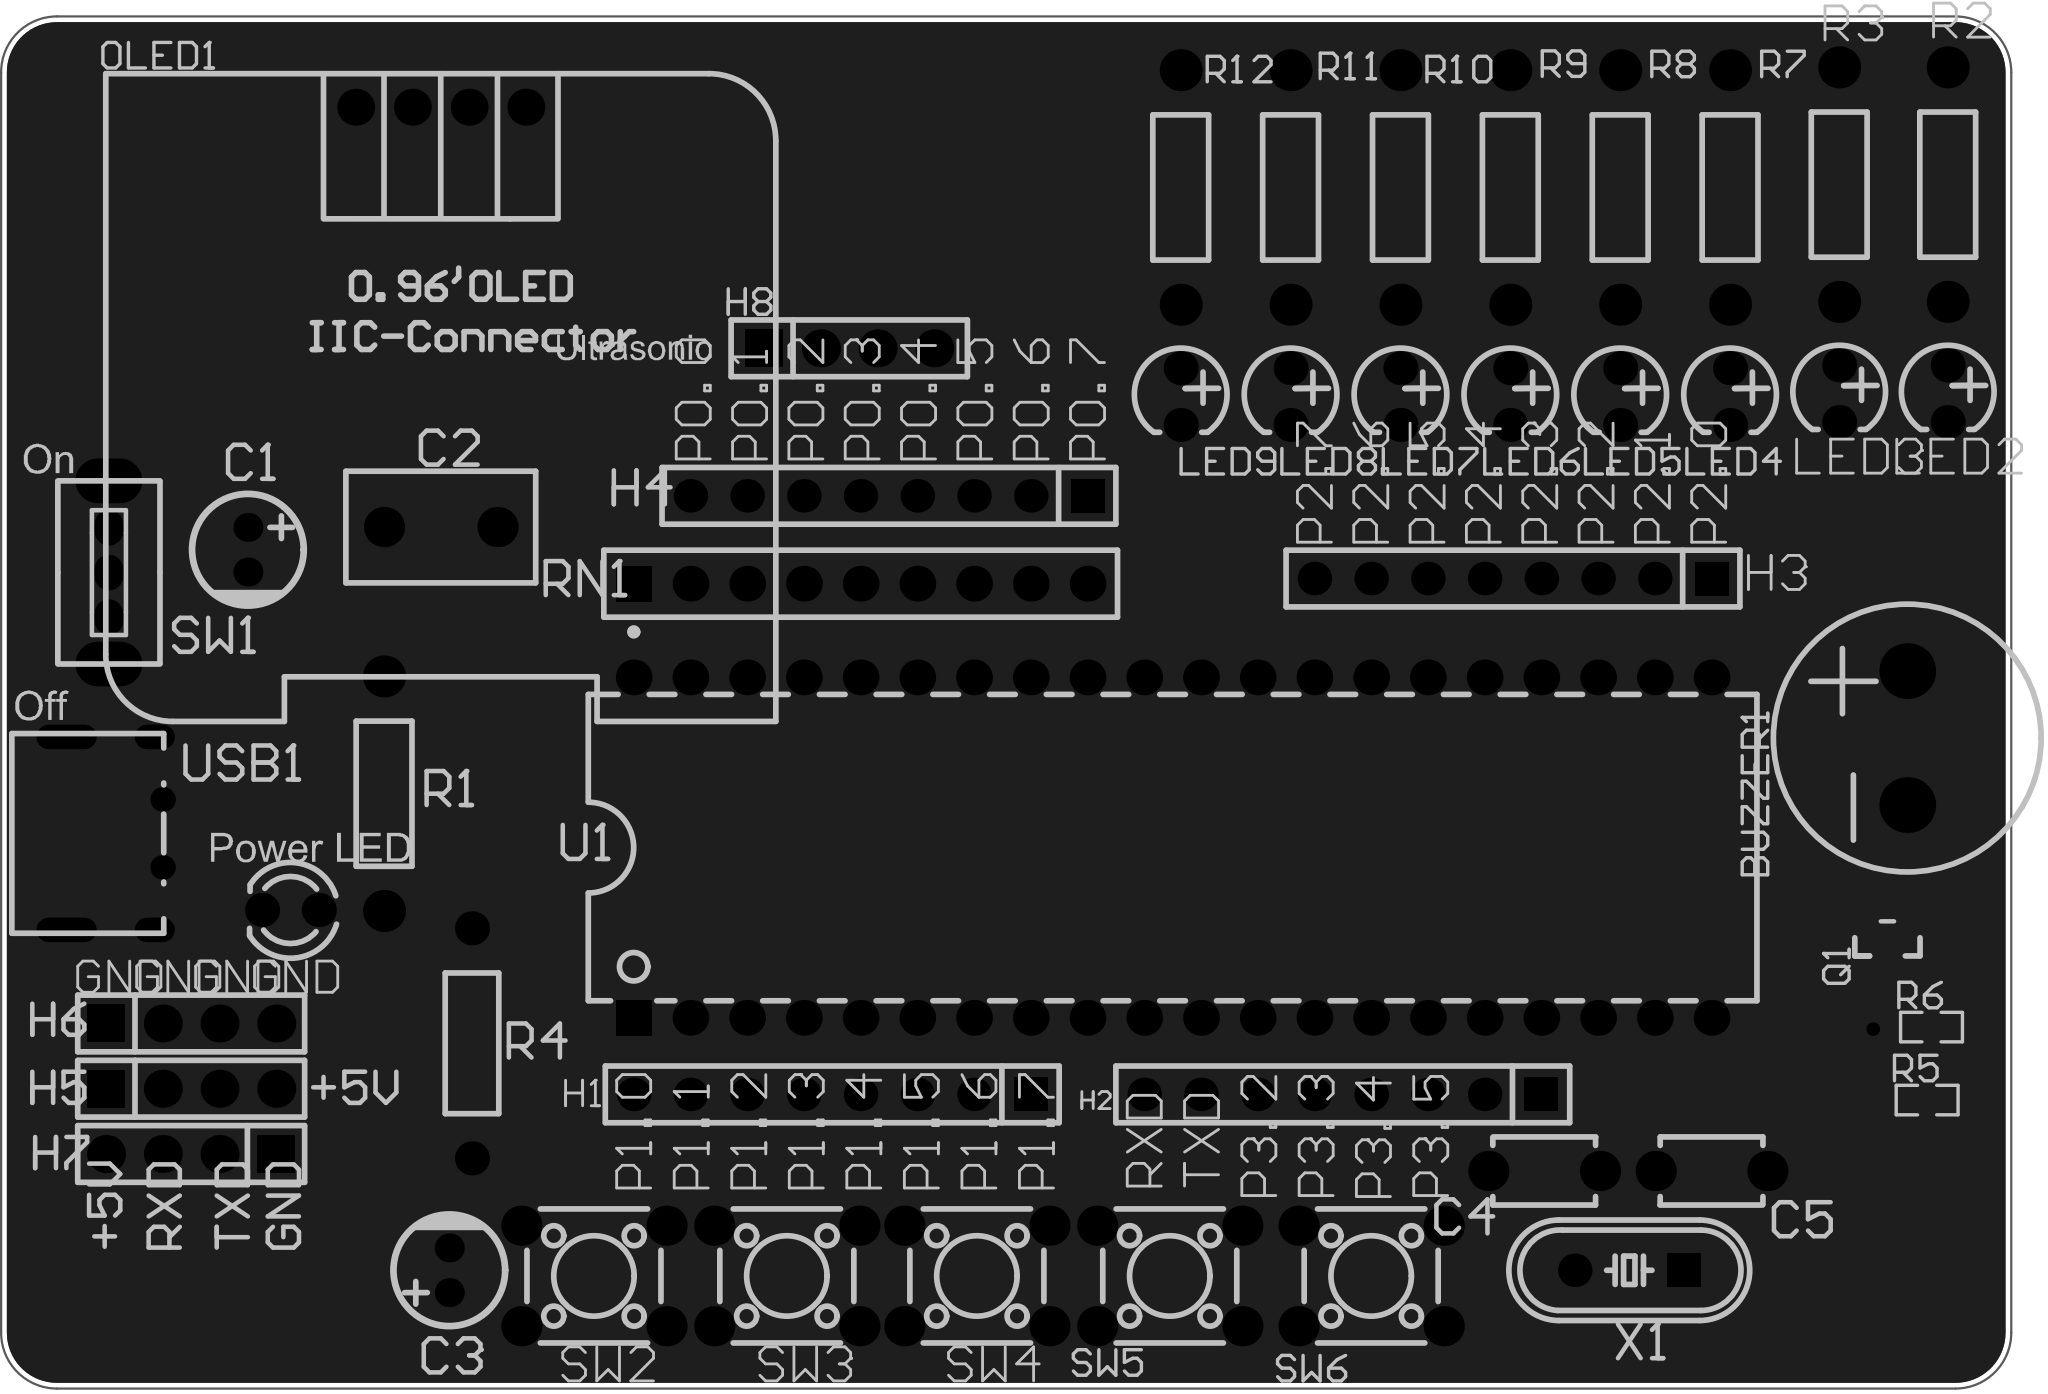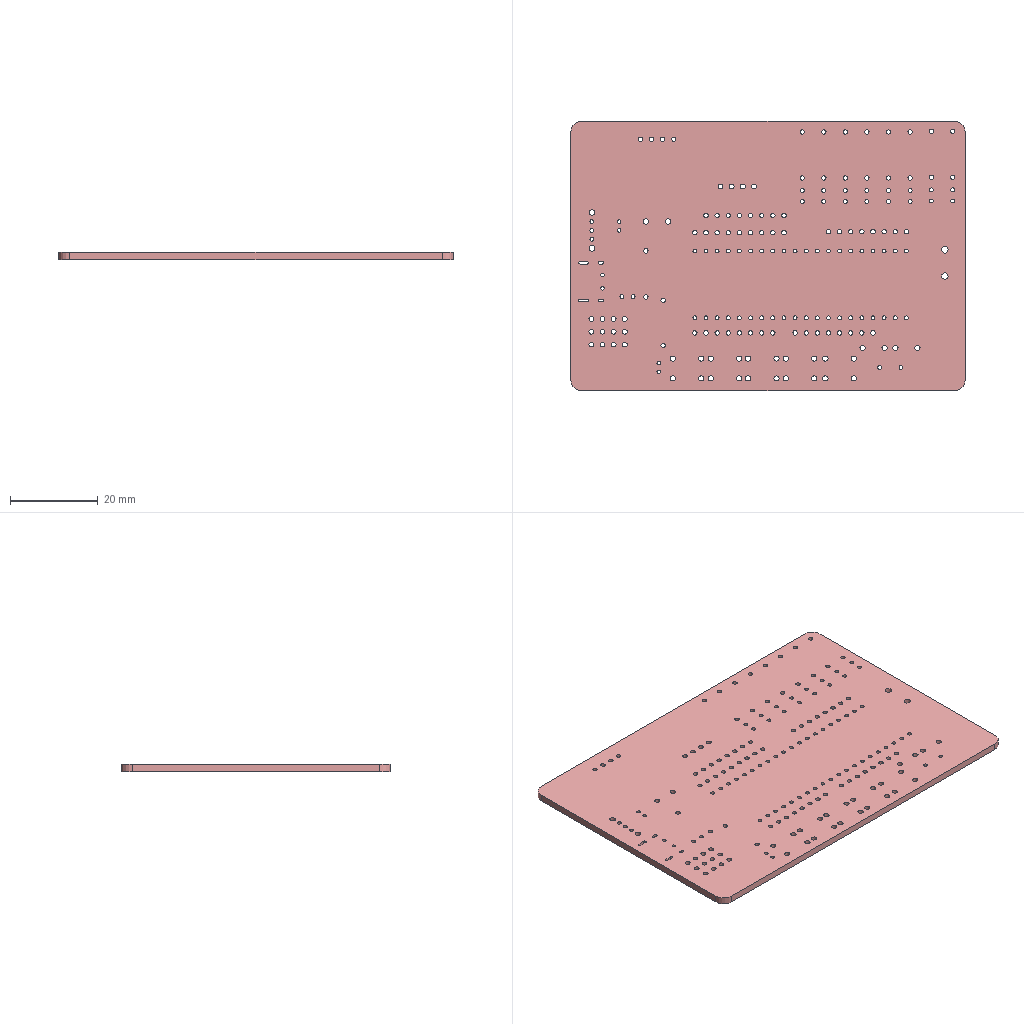Circuit board layout | Altium Designer | box 90 x 61.4 x 1.6 mm
Layer stack:
# Altium Designer layer stack of  (unit mm; dielectric type: 0 none, 1 core, 2 prepreg, 3 surface material)
index,name,kind,layer,copper_thickness_mm,dielectric_type,dielectric_thickness_mm,dielectric_material,dielectric_constant
0,Top Paste Mask Layer,other,,,,,,
1,Top Silkscreen Layer,other,,,,,,
2,Top Solder Mask Layer,dielectric,,,3,0.01,,3.3
3,Top Layer,copper,Top Layer,0.035,,,,
4,Dielectric1,dielectric,,,3,1.51,FR4,4.5
5,Bottom Layer,copper,Bottom Layer,0.035,,,,
6,Bottom Solder Mask Layer,dielectric,,,3,0.01,,3.3
7,Bottom Silkscreen Layer,other,,,,,,
8,Bottom Paste Mask Layer,other,,,,,,
# drill layer pairs: low layer,high layer
drill_pair,Top Layer,Bottom Layer
Part placement:
Designator,Comment,Layer,Footprint,Center-X(mm),Center-Y(mm),Rotation
U1,STC89C52RC-40I-PDIP40,TopLayer,DIP-40_L52.0-W13.7-P2.54-LS15.2-BL,128.651,100.457,0
SW3,,TopLayer,SW-TH_4P-L6.0-W6.0-P4.50-LS6.5,111.379,81.28,0
H8,,TopLayer,HDR-TH_4P-P2.54-V-F,114.173,122.809,0
SW4,,TopLayer,SW-TH_4P-L6.0-W6.0-P4.50-LS6.5,119.888,81.28,0
SW2,,TopLayer,SW-TH_4P-L6.0-W6.0-P4.50-LS6.5,102.743,81.28,180
RN1,10kΩ,TopLayer,RES-ARRAY-TH_9P-P2.54-D1.0,114.685,112.272,0
USB1,TYPE-C-31-M-33,TopLayer,USB-C-TH_TYPE-C-31-M-33,81.28,101.092,270
SW1,SS-12D02-VG4,TopLayer,SW-TH_SS-12D02-VG4,81.026,112.776,90
C1,10uF,TopLayer,CAP-TH_BD5.0-P2.00-D0.8-FD,87.249,113.792,270
R1,1kΩ,TopLayer,RES-TH_BD2.5-L6.5-P10.50-D0.6,93.345,102.87,270
LED1,204-10SURD/S530-A3-L,TopLayer,LED-TH_BD3.0-P2.54-FD,89.154,97.663,180
R2,1kΩ,TopLayer,RES-TH_BD2.5-L6.5-P10.50-D0.6,163.356,130.137,270
R3,1kΩ,TopLayer,RES-TH_BD2.5-L6.5-P10.50-D0.6,158.496,130.137,270
LED2,204-10SYGD/S530-E3,TopLayer,LED-TH_BD3.8-P2.54-FD,163.356,120.777,270
LED3,204-10SYGD/S530-E3,TopLayer,LED-TH_BD3.8-P2.54-FD,158.496,120.777,270
H1,,TopLayer,HDR-TH_8P-P2.54-V-M,113.411,89.408,180
H2,,TopLayer,HDR-TH_8P-P2.54-V-M,136.271,89.408,180
H3,,TopLayer,HDR-TH_8P-P2.54-V-M,143.891,112.502,180
H4,,TopLayer,HDR-TH_8P-P2.54-V-M,115.951,116.205,180
H7,,TopLayer,HDR-TH_4P-P2.54-V-M,84.709,86.741,180
H5,,TopLayer,HDR-TH_4P-P2.54-V-M,84.709,89.662,0
H6,,TopLayer,HDR-TH_4P-P2.54-V-M,84.709,92.583,0
C2,100nF,TopLayer,CAP-TH_L8.5-W5.0-P5.00-D1.2,95.885,114.808,180
C4,47pF,TopLayer,CAP-TH_L4.5-W3.0-P5.00-D1.2,145.288,85.979,0
C5,47pF,TopLayer,CAP-TH_L4.5-W3.0-P5.00-D1.2,152.781,85.979,180
X1,11.059MHz,TopLayer,HC-49US_L11.5-W4.5-P4.88,149.098,81.534,180
C3,10uF,TopLayer,CAP-TH_BD5.0-P2.00-D0.8-FD,96.266,81.534,90
R4,10kΩ,TopLayer,RES-TH_BD2.4-L6.3-P10.30-D0.6,97.282,91.694,270
BUZZER1,buzzer,TopLayer,BUZ-TH_BD12.0-P6.00-D0.9-RD,161.544,105.361,90
LED4,204-10SYGD/S530-E3,TopLayer,LED-TH_BD3.8-P2.54-FD,153.61,120.65,270
LED5,204-10SYGD/S530-E3,TopLayer,LED-TH_BD3.8-P2.54-FD,148.691,120.65,270
LED6,204-10SYGD/S530-E3,TopLayer,LED-TH_BD3.8-P2.54-FD,143.772,120.65,270
LED7,204-10SYGD/S530-E3,TopLayer,LED-TH_BD3.8-P2.54-FD,138.852,120.65,270
LED8,204-10SYGD/S530-E3,TopLayer,LED-TH_BD3.8-P2.54-FD,133.933,120.65,270
LED9,204-10SYGD/S530-E3,TopLayer,LED-TH_BD3.8-P2.54-FD,129.014,120.65,270
OLED1,,TopLayer,0.96OLED_4P,95.885,133.604,0
Q1,,TopLayer,S8550P_SOT,160.655,96.257,90
R5,1K,TopLayer,R0603,162.433,89.154,0
R6,1K,TopLayer,R0603,162.629,92.421,0
R7,1kΩ,TopLayer,RES-TH_BD2.5-L6.5-P10.50-D0.6,153.61,130.01,270
R8,1kΩ,TopLayer,RES-TH_BD2.5-L6.5-P10.50-D0.6,148.691,130.01,270
R9,1kΩ,TopLayer,RES-TH_BD2.5-L6.5-P10.50-D0.6,143.772,130.01,270
R10,1kΩ,TopLayer,RES-TH_BD2.5-L6.5-P10.50-D0.6,138.852,130.01,270
R11,1kΩ,TopLayer,RES-TH_BD2.5-L6.5-P10.50-D0.6,133.933,130.01,270
R12,1kΩ,TopLayer,RES-TH_BD2.5-L6.5-P10.50-D0.6,129.014,130.01,270
SW5,,TopLayer,SW-TH_4P-L6.0-W6.0-P4.50-LS6.5,128.524,81.28,0
SW6,,TopLayer,SW-TH_4P-L6.0-W6.0-P4.50-LS6.5,137.541,81.28,0
Pad and via stacks:
# Altium Designer via and pad stacks of  (unit mm). Each distinct definition once, with the count of objects using it.
# via: kind,start_layer,end_layer,hole_mm,diameter_mm,mode(0 simple;1 top-mid-bottom;2 full stack),diameter_per_layer,count,example_net
# pad: kind,layer,hole_mm,hole_type(0 round;1 square;2 slot),plating,top_size,top_shape(1 round;2 rect;3 octagon;9 rounded rect),mid_size,bottom_size,mode,footprint,size_per_layer,count,example
pad,Multi-Layer,0.889,0,plated,1.6x1.6,1,1.6x1.6,1.6x1.6,0,DIP-40_L52.0-W13.7-P2.54-LS15.2-BL,,39,U1.31
pad,Multi-Layer,0.889,0,plated,1.6x1.6,2,1.6x1.6,1.6x1.6,0,DIP-40_L52.0-W13.7-P2.54-LS15.2-BL,,1,U1.1
pad,Multi-Layer,1.2,0,plated,1.8x1.8,1,1.8x1.8,1.8x1.8,0,SW-TH_4P-L6.0-W6.0-P4.50-LS6.5,,20,SW3.1
pad,Multi-Layer,1.1,0,plated,1.7x1.7,2,1.7x1.7,1.7x1.7,0,HDR-TH_4P-P2.54-V-F,,1,H8.1
pad,Multi-Layer,1.1,0,plated,1.7x1.7,1,1.7x1.7,1.7x1.7,0,HDR-TH_4P-P2.54-V-F,,3,H8.2
pad,Multi-Layer,1,0,plated,1.6x1.6,2,1.6x1.6,1.6x1.6,0,RES-ARRAY-TH_9P-P2.54-D1.0,,1,RN1.1
pad,Multi-Layer,1,0,plated,1.6x1.6,1,1.6x1.6,1.6x1.6,0,RES-ARRAY-TH_9P-P2.54-D1.0,,8,RN1.2
pad,Multi-Layer,0.8,0,plated,1.1x1.1,1,1.1x1.1,1.1x1.1,0,USB-C-TH_TYPE-C-31-M-33,,2,USB1.B12
pad,Multi-Layer,0.6,2,plated,1.8x1.1,1,1.8x1.1,1.8x1.1,0,USB-C-TH_TYPE-C-31-M-33,,2,USB1.3
pad,Multi-Layer,0.6,2,plated,1.1x2.7,1,1.1x2.7,1.1x2.7,0,USB-C-TH_TYPE-C-31-M-33,,2,USB1.4
pad,Multi-Layer,0.9,0,plated,1.6x1.3,1,1.6x1.3,1.6x1.3,0,SW-TH_SS-12D02-VG4,,3,SW1.1
pad,Multi-Layer,1.3,0,plated,3x2,1,3x2,3x2,0,SW-TH_SS-12D02-VG4,,2,SW1.4
pad,Multi-Layer,0.8,0,plated,1.3x1.3,1,1.3x1.3,1.3x1.3,0,CAP-TH_BD5.0-P2.00-D0.8-FD,,4,C1.1
pad,Multi-Layer,1,0,plated,1.88x1.88,1,1.88x1.88,1.88x1.88,0,RES-TH_BD2.5-L6.5-P10.50-D0.6,,18,R1.1
pad,Multi-Layer,0.9144,0,plated,1.524x1.524,1,1.524x1.524,1.524x1.524,0,LED-TH_BD3.0-P2.54-FD,,2,LED1.1
pad,Multi-Layer,0.9,0,plated,1.524x1.524,1,1.524x1.524,1.524x1.524,0,LED-TH_BD3.8-P2.54-FD,,16,LED2.2
pad,Multi-Layer,1,0,plated,1.5x1.5,2,1.5x1.5,1.5x1.5,0,HDR-TH_8P-P2.54-V-M,,4,H1.1
pad,Multi-Layer,1,0,plated,1.5x1.5,1,1.5x1.5,1.5x1.5,0,HDR-TH_8P-P2.54-V-M,,28,H1.2
pad,Multi-Layer,1.1,0,plated,1.7x1.7,2,1.7x1.7,1.7x1.7,0,HDR-TH_4P-P2.54-V-M,,3,H7.1
pad,Multi-Layer,1.1,0,plated,1.7x1.7,1,1.7x1.7,1.7x1.7,0,HDR-TH_4P-P2.54-V-M,,9,H7.2
pad,Multi-Layer,1.2,0,plated,1.8x1.8,1,1.8x1.8,1.8x1.8,0,CAP-TH_L8.5-W5.0-P5.00-D1.2,,2,C2.1
pad,Multi-Layer,1.2,0,plated,1.8x1.8,1,1.8x1.8,1.8x1.8,0,CAP-TH_L4.5-W3.0-P5.00-D1.2,,4,C4.1
pad,Multi-Layer,0.9,0,plated,1.5x1.5,2,1.5x1.5,1.5x1.5,0,HC-49US_L11.5-W4.5-P4.88,,1,X1.1
pad,Multi-Layer,0.9,0,plated,1.5x1.5,1,1.5x1.5,1.5x1.5,0,HC-49US_L11.5-W4.5-P4.88,,1,X1.2
pad,Multi-Layer,1,0,plated,1.524x1.524,1,1.524x1.524,1.524x1.524,0,RES-TH_BD2.4-L6.3-P10.30-D0.6,,2,R4.1
pad,Multi-Layer,1.5,0,plated,2.5x2.5,1,2.5x2.5,2.5x2.5,0,BUZ-TH_BD12.0-P6.00-D0.9-RD,,2,BUZZER1.1
pad,Multi-Layer,1,0,plated,1.65x1.65,1,1.65x1.65,1.65x1.65,0,0.96OLED_4P,,4,OLED1.4
pad,Top Layer,0,0,plated,0.701x1.25,2,0.701x1.25,0.701x1.25,0,S8550P_SOT,,3,Q1.3
pad,Top Layer,0,0,plated,0.8065x0.864,2,0.8065x0.864,0.8065x0.864,0,R0603,,4,R5.2
via,Top Layer,Bottom Layer,0.3048,0.6096,0,,1,P1.5
Copper pours:
name,layer,net,type(0 solid;1 hatched;2 none)
Top Layer-GND,Top Layer,GND,0
Bottom Layer-GND,Bottom Layer,GND,0
Design rules, without the lines most boards share:
# Altium Designer design rules of  (exported by Altium Designer, unit mm)
# columns: name | kind | enabled | priority | scope1 | scope2 | descriptor | typed fields (field=value)
copperThickness2oz | 0 | disabled | 1 | All | All | Clearance Constraint (Gap=6mil) (Disabled)(All),(All) | gap=0.1524
otherClearance | 52 | enabled | 1 | All | All | Hole To Hole Clearance (Gap=11.8mil) (All),(All) | gap=0.2997
viaSize | 11 | enabled | 1 | All | All | Routing Via (MinHoleWidth=11.8mil) (MaxHoleWidth=248mil) (PreferredHoleWidth=12mil) (MinWidth=19.7mil) (MaxWidth=393.7mil) (PreferedWidth=24mil) (All) | via_min_hole=0.2997 via_max_hole=6.299 via_preferred_diameter=0.6096 via_preferred_hole=0.3048